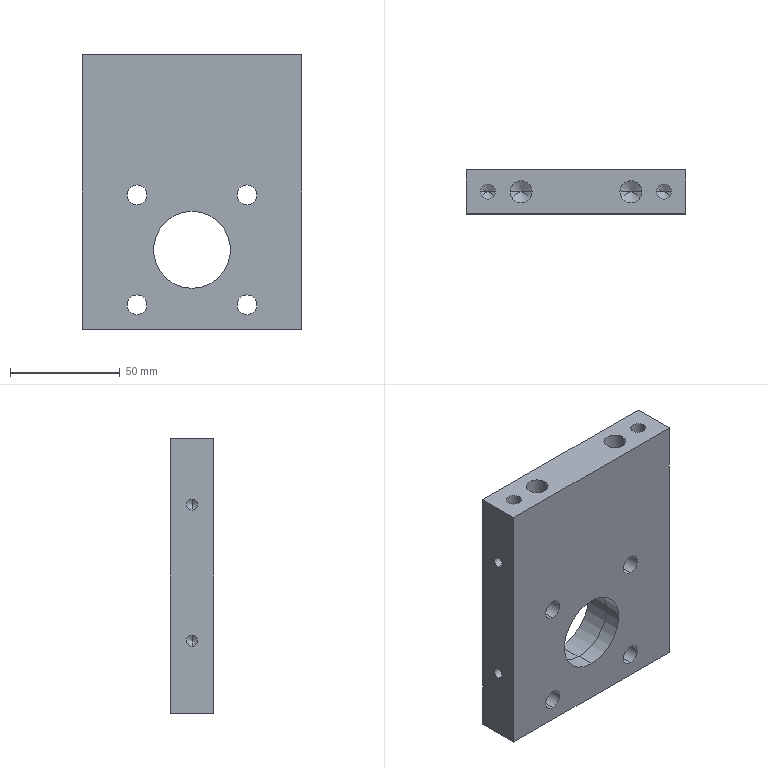Part | STEP file | OP10-131_cylinder stand (2) -L | 1 solid | 63 faces | box 100 x 20 x 125 mm | volume 216562 mm3 | cylinder 36 | cone 16 | plane 11 | commonest cylinder face diameters 5 x8 9 x8 14 x8 6.8 x4 10 x4 35 x2